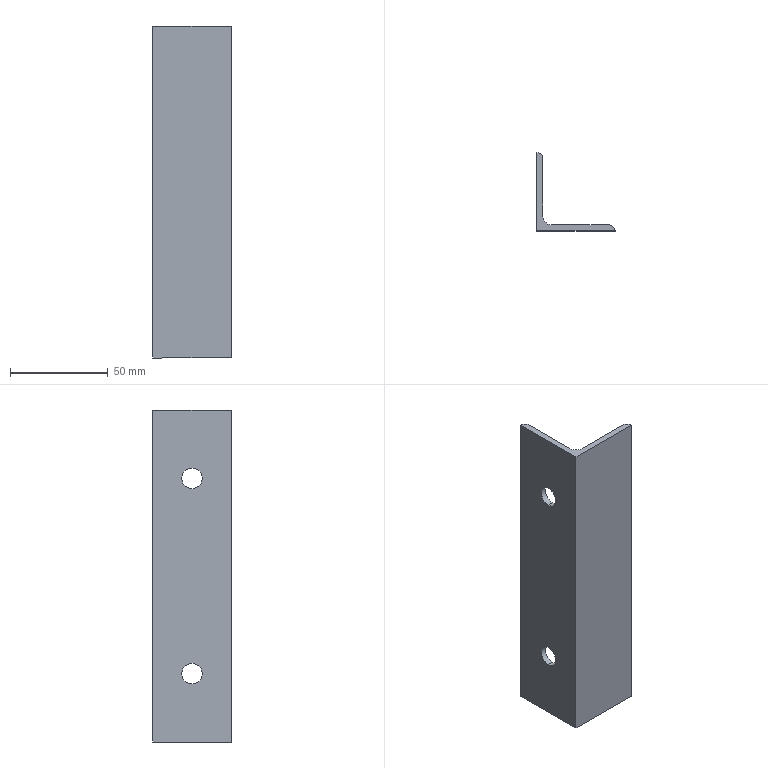Part | SolidWorks | features BaseBody 1 | 1 solid | 13 faces | box 40 x 40 x 170 mm | volume 38833 mm3 | cylinder 7 | plane 6 | commonest cylinder face diameters 10.5 x4 6 x2 9 x1
STEP:
#1=CARTESIAN_POINT('',(3.,20.,-55.25));
#2=VERTEX_POINT('',#1);
#3=CARTESIAN_POINT('',(0.,20.,-55.25));
#4=VERTEX_POINT('',#3);
#5=CARTESIAN_POINT('',(10.,20.,-55.25));
#6=DIRECTION('',(-1.,0.,0.));
#7=VECTOR('',#6,1000.);
#8=LINE('',#5,#7);
#9=EDGE_CURVE('',#2,#4,#8,.T.);
#10=ORIENTED_EDGE('',*,*,#9,.F.);
#11=CARTESIAN_POINT('',(3.,20.,-44.75));
#12=VERTEX_POINT('',#11);
#13=CARTESIAN_POINT('',(3.,20.,-50.));
#14=DIRECTION('',(-1.,0.,0.));
#15=DIRECTION('',(0.,-1.,0.));
#16=AXIS2_PLACEMENT_3D('',#13,#14,#15);
#17=CIRCLE('',#16,5.25);
#18=EDGE_CURVE('',#12,#2,#17,.T.);
#19=ORIENTED_EDGE('',*,*,#18,.F.);
#20=CARTESIAN_POINT('',(0.,20.,-44.75));
#21=VERTEX_POINT('',#20);
#22=CARTESIAN_POINT('',(10.,20.,-44.75));
#23=DIRECTION('',(-1.,0.,0.));
#24=VECTOR('',#23,1000.);
#25=LINE('',#22,#24);
#26=EDGE_CURVE('',#12,#21,#25,.T.);
#27=ORIENTED_EDGE('',*,*,#26,.T.);
#28=CARTESIAN_POINT('',(0.,20.,-50.));
#29=DIRECTION('',(-1.,0.,0.));
#30=DIRECTION('',(0.,0.,1.));
#31=AXIS2_PLACEMENT_3D('',#28,#29,#30);
#32=CIRCLE('',#31,5.25);
#33=EDGE_CURVE('',#21,#4,#32,.T.);
#34=ORIENTED_EDGE('',*,*,#33,.T.);
#35=EDGE_LOOP('',(#10,#19,#27,#34));
#36=FACE_OUTER_BOUND('',#35,.T.);
#37=CARTESIAN_POINT('',(10.,20.,-50.));
#38=DIRECTION('',(-1.,0.,0.));
#39=DIRECTION('',(0.,0.,1.));
#40=AXIS2_PLACEMENT_3D('',#37,#38,#39);
#41=CYLINDRICAL_SURFACE('',#40,5.25);
#42=ADVANCED_FACE('',(#36),#41,.F.);
#43=CARTESIAN_POINT('',(3.,20.,44.75));
#44=VERTEX_POINT('',#43);
#45=CARTESIAN_POINT('',(0.,20.,44.75));
#46=VERTEX_POINT('',#45);
#47=CARTESIAN_POINT('',(10.,20.,44.75));
#48=DIRECTION('',(-1.,0.,0.));
#49=VECTOR('',#48,1000.);
#50=LINE('',#47,#49);
#51=EDGE_CURVE('',#44,#46,#50,.T.);
#52=ORIENTED_EDGE('',*,*,#51,.F.);
#53=CARTESIAN_POINT('',(3.,20.,55.25));
#54=VERTEX_POINT('',#53);
#55=CARTESIAN_POINT('',(3.,20.,50.));
#56=DIRECTION('',(-1.,0.,0.));
#57=DIRECTION('',(0.,-1.,0.));
#58=AXIS2_PLACEMENT_3D('',#55,#56,#57);
#59=CIRCLE('',#58,5.25);
#60=EDGE_CURVE('',#54,#44,#59,.T.);
#61=ORIENTED_EDGE('',*,*,#60,.F.);
#62=CARTESIAN_POINT('',(0.,20.,55.25));
#63=VERTEX_POINT('',#62);
#64=CARTESIAN_POINT('',(10.,20.,55.25));
#65=DIRECTION('',(-1.,0.,0.));
#66=VECTOR('',#65,1000.);
#67=LINE('',#64,#66);
#68=EDGE_CURVE('',#54,#63,#67,.T.);
#69=ORIENTED_EDGE('',*,*,#68,.T.);
#70=CARTESIAN_POINT('',(0.,20.,50.));
#71=DIRECTION('',(-1.,0.,0.));
#72=DIRECTION('',(0.,0.,-1.));
#73=AXIS2_PLACEMENT_3D('',#70,#71,#72);
#74=CIRCLE('',#73,5.25);
#75=EDGE_CURVE('',#63,#46,#74,.T.);
#76=ORIENTED_EDGE('',*,*,#75,.T.);
#77=EDGE_LOOP('',(#52,#61,#69,#76));
#78=FACE_OUTER_BOUND('',#77,.T.);
#79=CARTESIAN_POINT('',(10.,20.,50.));
#80=DIRECTION('',(-1.,0.,0.));
#81=DIRECTION('',(0.,0.,1.));
#82=AXIS2_PLACEMENT_3D('',#79,#80,#81);
#83=CYLINDRICAL_SURFACE('',#82,5.25);
#84=ADVANCED_FACE('',(#78),#83,.F.);
#85=CARTESIAN_POINT('',(3.,37.,85.));
#86=VERTEX_POINT('',#85);
#87=CARTESIAN_POINT('',(0.,40.,85.));
#88=VERTEX_POINT('',#87);
#89=CARTESIAN_POINT('',(0.,37.,85.));
#90=DIRECTION('',(0.,0.,1.));
#91=DIRECTION('',(-1.,0.,0.));
#92=AXIS2_PLACEMENT_3D('',#89,#90,#91);
#93=CIRCLE('',#92,3.);
#94=EDGE_CURVE('',#86,#88,#93,.T.);
#95=ORIENTED_EDGE('',*,*,#94,.F.);
#96=CARTESIAN_POINT('',(3.,37.,-85.));
#97=VERTEX_POINT('',#96);
#98=CARTESIAN_POINT('',(3.,37.,85.));
#99=DIRECTION('',(0.,0.,1.));
#100=VECTOR('',#99,1000.);
#101=LINE('',#98,#100);
#102=EDGE_CURVE('',#97,#86,#101,.T.);
#103=ORIENTED_EDGE('',*,*,#102,.F.);
#104=CARTESIAN_POINT('',(0.,40.,-85.));
#105=VERTEX_POINT('',#104);
#106=CARTESIAN_POINT('',(0.,37.,-85.));
#107=DIRECTION('',(0.,0.,-1.));
#108=DIRECTION('',(-1.,0.,0.));
#109=AXIS2_PLACEMENT_3D('',#106,#107,#108);
#110=CIRCLE('',#109,3.);
#111=EDGE_CURVE('',#105,#97,#110,.T.);
#112=ORIENTED_EDGE('',*,*,#111,.F.);
#113=CARTESIAN_POINT('',(0.,40.,85.));
#114=DIRECTION('',(0.,0.,-1.));
#115=VECTOR('',#114,1000.);
#116=LINE('',#113,#115);
#117=EDGE_CURVE('',#88,#105,#116,.T.);
#118=ORIENTED_EDGE('',*,*,#117,.F.);
#119=EDGE_LOOP('',(#95,#103,#112,#118));
#120=FACE_OUTER_BOUND('',#119,.T.);
#121=CARTESIAN_POINT('',(0.,37.,85.));
#122=DIRECTION('',(0.,0.,-1.));
#123=DIRECTION('',(-1.,0.,0.));
#124=AXIS2_PLACEMENT_3D('',#121,#122,#123);
#125=CYLINDRICAL_SURFACE('',#124,3.);
#126=ADVANCED_FACE('',(#120),#125,.T.);
#127=CARTESIAN_POINT('',(40.,0.,85.));
#128=VERTEX_POINT('',#127);
#129=CARTESIAN_POINT('',(37.,3.,85.));
#130=VERTEX_POINT('',#129);
#131=CARTESIAN_POINT('',(37.,0.,85.));
#132=DIRECTION('',(0.,0.,1.));
#133=DIRECTION('',(-1.,0.,0.));
#134=AXIS2_PLACEMENT_3D('',#131,#132,#133);
#135=CIRCLE('',#134,3.);
#136=EDGE_CURVE('',#128,#130,#135,.T.);
#137=ORIENTED_EDGE('',*,*,#136,.F.);
#138=CARTESIAN_POINT('',(40.,0.,-85.));
#139=VERTEX_POINT('',#138);
#140=CARTESIAN_POINT('',(40.,0.,85.));
#141=DIRECTION('',(0.,0.,-1.));
#142=VECTOR('',#141,1000.);
#143=LINE('',#140,#142);
#144=EDGE_CURVE('',#128,#139,#143,.T.);
#145=ORIENTED_EDGE('',*,*,#144,.T.);
#146=CARTESIAN_POINT('',(37.,3.,-85.));
#147=VERTEX_POINT('',#146);
#148=CARTESIAN_POINT('',(37.,0.,-85.));
#149=DIRECTION('',(0.,0.,-1.));
#150=DIRECTION('',(-1.,0.,0.));
#151=AXIS2_PLACEMENT_3D('',#148,#149,#150);
#152=CIRCLE('',#151,3.);
#153=EDGE_CURVE('',#147,#139,#152,.T.);
#154=ORIENTED_EDGE('',*,*,#153,.F.);
#155=CARTESIAN_POINT('',(37.,3.,85.));
#156=DIRECTION('',(0.,0.,-1.));
#157=VECTOR('',#156,1000.);
#158=LINE('',#155,#157);
#159=EDGE_CURVE('',#130,#147,#158,.T.);
#160=ORIENTED_EDGE('',*,*,#159,.F.);
#161=EDGE_LOOP('',(#137,#145,#154,#160));
#162=FACE_OUTER_BOUND('',#161,.T.);
#163=CARTESIAN_POINT('',(37.,0.,85.));
#164=DIRECTION('',(0.,0.,-1.));
#165=DIRECTION('',(-1.,0.,0.));
#166=AXIS2_PLACEMENT_3D('',#163,#164,#165);
#167=CYLINDRICAL_SURFACE('',#166,3.);
#168=ADVANCED_FACE('',(#162),#167,.T.);
#169=CARTESIAN_POINT('',(7.5,3.,85.));
#170=VERTEX_POINT('',#169);
#171=CARTESIAN_POINT('',(3.,7.5,85.));
#172=VERTEX_POINT('',#171);
#173=CARTESIAN_POINT('',(7.5,7.5,85.));
#174=DIRECTION('',(0.,0.,-1.));
#175=DIRECTION('',(-1.,0.,0.));
#176=AXIS2_PLACEMENT_3D('',#173,#174,#175);
#177=CIRCLE('',#176,4.5);
#178=EDGE_CURVE('',#170,#172,#177,.T.);
#179=ORIENTED_EDGE('',*,*,#178,.F.);
#180=CARTESIAN_POINT('',(7.5,3.,-85.));
#181=VERTEX_POINT('',#180);
#182=CARTESIAN_POINT('',(7.5,3.,85.));
#183=DIRECTION('',(0.,0.,1.));
#184=VECTOR('',#183,1000.);
#185=LINE('',#182,#184);
#186=EDGE_CURVE('',#181,#170,#185,.T.);
#187=ORIENTED_EDGE('',*,*,#186,.F.);
#188=CARTESIAN_POINT('',(3.,7.5,-85.));
#189=VERTEX_POINT('',#188);
#190=CARTESIAN_POINT('',(7.5,7.5,-85.));
#191=DIRECTION('',(0.,0.,1.));
#192=DIRECTION('',(-1.,0.,0.));
#193=AXIS2_PLACEMENT_3D('',#190,#191,#192);
#194=CIRCLE('',#193,4.5);
#195=EDGE_CURVE('',#189,#181,#194,.T.);
#196=ORIENTED_EDGE('',*,*,#195,.F.);
#197=CARTESIAN_POINT('',(3.,7.5,-85.));
#198=DIRECTION('',(0.,0.,-1.));
#199=VECTOR('',#198,1000.);
#200=LINE('',#197,#199);
#201=EDGE_CURVE('',#172,#189,#200,.T.);
#202=ORIENTED_EDGE('',*,*,#201,.F.);
#203=EDGE_LOOP('',(#179,#187,#196,#202));
#204=FACE_OUTER_BOUND('',#203,.T.);
#205=CARTESIAN_POINT('',(7.5,7.5,85.));
#206=DIRECTION('',(0.,0.,1.));
#207=DIRECTION('',(1.,0.,0.));
#208=AXIS2_PLACEMENT_3D('',#205,#206,#207);
#209=CYLINDRICAL_SURFACE('',#208,4.5);
#210=ADVANCED_FACE('',(#204),#209,.F.);
#211=CARTESIAN_POINT('',(3.,3.,-85.));
#212=DIRECTION('',(-1.,0.,0.));
#213=VECTOR('',#212,1000.);
#214=LINE('',#211,#213);
#215=EDGE_CURVE('',#147,#181,#214,.T.);
#216=ORIENTED_EDGE('',*,*,#215,.F.);
#217=ORIENTED_EDGE('',*,*,#153,.T.);
#218=CARTESIAN_POINT('',(0.,0.,-85.));
#219=VERTEX_POINT('',#218);
#220=CARTESIAN_POINT('',(0.,0.,-85.));
#221=DIRECTION('',(1.,0.,0.));
#222=VECTOR('',#221,1000.);
#223=LINE('',#220,#222);
#224=EDGE_CURVE('',#219,#139,#223,.T.);
#225=ORIENTED_EDGE('',*,*,#224,.F.);
#226=CARTESIAN_POINT('',(0.,0.,-85.));
#227=DIRECTION('',(0.,-1.,0.));
#228=VECTOR('',#227,1000.);
#229=LINE('',#226,#228);
#230=EDGE_CURVE('',#105,#219,#229,.T.);
#231=ORIENTED_EDGE('',*,*,#230,.F.);
#232=ORIENTED_EDGE('',*,*,#111,.T.);
#233=CARTESIAN_POINT('',(3.,40.,-85.));
#234=DIRECTION('',(0.,1.,0.));
#235=VECTOR('',#234,1000.);
#236=LINE('',#233,#235);
#237=EDGE_CURVE('',#189,#97,#236,.T.);
#238=ORIENTED_EDGE('',*,*,#237,.F.);
#239=ORIENTED_EDGE('',*,*,#195,.T.);
#240=EDGE_LOOP('',(#216,#217,#225,#231,#232,#238,#239));
#241=FACE_OUTER_BOUND('',#240,.T.);
#242=CARTESIAN_POINT('',(0.,0.,-85.));
#243=DIRECTION('',(0.,0.,-1.));
#244=DIRECTION('',(0.,-1.,0.));
#245=AXIS2_PLACEMENT_3D('',#242,#243,#244);
#246=PLANE('',#245);
#247=ADVANCED_FACE('',(#241),#246,.T.);
#248=CARTESIAN_POINT('',(0.,0.,85.));
#249=VERTEX_POINT('',#248);
#250=CARTESIAN_POINT('',(0.,0.,85.));
#251=DIRECTION('',(1.,0.,0.));
#252=VECTOR('',#251,1000.);
#253=LINE('',#250,#252);
#254=EDGE_CURVE('',#249,#128,#253,.T.);
#255=ORIENTED_EDGE('',*,*,#254,.T.);
#256=ORIENTED_EDGE('',*,*,#136,.T.);
#257=CARTESIAN_POINT('',(3.,3.,85.));
#258=DIRECTION('',(-1.,0.,0.));
#259=VECTOR('',#258,1000.);
#260=LINE('',#257,#259);
#261=EDGE_CURVE('',#130,#170,#260,.T.);
#262=ORIENTED_EDGE('',*,*,#261,.T.);
#263=ORIENTED_EDGE('',*,*,#178,.T.);
#264=CARTESIAN_POINT('',(3.,40.,85.));
#265=DIRECTION('',(0.,1.,0.));
#266=VECTOR('',#265,1000.);
#267=LINE('',#264,#266);
#268=EDGE_CURVE('',#172,#86,#267,.T.);
#269=ORIENTED_EDGE('',*,*,#268,.T.);
#270=ORIENTED_EDGE('',*,*,#94,.T.);
#271=CARTESIAN_POINT('',(0.,0.,85.));
#272=DIRECTION('',(0.,-1.,0.));
#273=VECTOR('',#272,1000.);
#274=LINE('',#271,#273);
#275=EDGE_CURVE('',#88,#249,#274,.T.);
#276=ORIENTED_EDGE('',*,*,#275,.T.);
#277=EDGE_LOOP('',(#255,#256,#262,#263,#269,#270,#276));
#278=FACE_OUTER_BOUND('',#277,.T.);
#279=CARTESIAN_POINT('',(0.,0.,85.));
#280=DIRECTION('',(0.,0.,-1.));
#281=DIRECTION('',(0.,-1.,0.));
#282=AXIS2_PLACEMENT_3D('',#279,#280,#281);
#283=PLANE('',#282);
#284=ADVANCED_FACE('',(#278),#283,.F.);
#285=ORIENTED_EDGE('',*,*,#60,.T.);
#286=CARTESIAN_POINT('',(3.,20.,50.));
#287=DIRECTION('',(-1.,0.,0.));
#288=DIRECTION('',(0.,-1.,0.));
#289=AXIS2_PLACEMENT_3D('',#286,#287,#288);
#290=CIRCLE('',#289,5.25);
#291=EDGE_CURVE('',#44,#54,#290,.T.);
#292=ORIENTED_EDGE('',*,*,#291,.T.);
#293=EDGE_LOOP('',(#285,#292));
#294=FACE_BOUND('',#293,.T.);
#295=ORIENTED_EDGE('',*,*,#18,.T.);
#296=CARTESIAN_POINT('',(3.,20.,-50.));
#297=DIRECTION('',(-1.,0.,0.));
#298=DIRECTION('',(0.,-1.,0.));
#299=AXIS2_PLACEMENT_3D('',#296,#297,#298);
#300=CIRCLE('',#299,5.25);
#301=EDGE_CURVE('',#2,#12,#300,.T.);
#302=ORIENTED_EDGE('',*,*,#301,.T.);
#303=EDGE_LOOP('',(#295,#302));
#304=FACE_BOUND('',#303,.T.);
#305=ORIENTED_EDGE('',*,*,#237,.T.);
#306=ORIENTED_EDGE('',*,*,#102,.T.);
#307=ORIENTED_EDGE('',*,*,#268,.F.);
#308=ORIENTED_EDGE('',*,*,#201,.T.);
#309=EDGE_LOOP('',(#305,#306,#307,#308));
#310=FACE_OUTER_BOUND('',#309,.T.);
#311=CARTESIAN_POINT('',(3.,40.,85.));
#312=DIRECTION('',(-1.,0.,0.));
#313=DIRECTION('',(0.,1.,0.));
#314=AXIS2_PLACEMENT_3D('',#311,#312,#313);
#315=PLANE('',#314);
#316=ADVANCED_FACE('',(#294,#304,#310),#315,.F.);
#317=ORIENTED_EDGE('',*,*,#261,.F.);
#318=ORIENTED_EDGE('',*,*,#159,.T.);
#319=ORIENTED_EDGE('',*,*,#215,.T.);
#320=ORIENTED_EDGE('',*,*,#186,.T.);
#321=EDGE_LOOP('',(#317,#318,#319,#320));
#322=FACE_OUTER_BOUND('',#321,.T.);
#323=CARTESIAN_POINT('',(3.,3.,85.));
#324=DIRECTION('',(0.,-1.,0.));
#325=DIRECTION('',(0.,0.,-1.));
#326=AXIS2_PLACEMENT_3D('',#323,#324,#325);
#327=PLANE('',#326);
#328=ADVANCED_FACE('',(#322),#327,.F.);
#329=ORIENTED_EDGE('',*,*,#224,.T.);
#330=ORIENTED_EDGE('',*,*,#144,.F.);
#331=ORIENTED_EDGE('',*,*,#254,.F.);
#332=CARTESIAN_POINT('',(0.,0.,85.));
#333=DIRECTION('',(0.,0.,-1.));
#334=VECTOR('',#333,1000.);
#335=LINE('',#332,#334);
#336=EDGE_CURVE('',#249,#219,#335,.T.);
#337=ORIENTED_EDGE('',*,*,#336,.T.);
#338=EDGE_LOOP('',(#329,#330,#331,#337));
#339=FACE_OUTER_BOUND('',#338,.T.);
#340=CARTESIAN_POINT('',(0.,0.,85.));
#341=DIRECTION('',(0.,1.,0.));
#342=DIRECTION('',(1.,0.,0.));
#343=AXIS2_PLACEMENT_3D('',#340,#341,#342);
#344=PLANE('',#343);
#345=ADVANCED_FACE('',(#339),#344,.F.);
#346=ORIENTED_EDGE('',*,*,#75,.F.);
#347=CARTESIAN_POINT('',(0.,20.,50.));
#348=DIRECTION('',(-1.,0.,0.));
#349=DIRECTION('',(0.,0.,-1.));
#350=AXIS2_PLACEMENT_3D('',#347,#348,#349);
#351=CIRCLE('',#350,5.25);
#352=EDGE_CURVE('',#46,#63,#351,.T.);
#353=ORIENTED_EDGE('',*,*,#352,.F.);
#354=EDGE_LOOP('',(#346,#353));
#355=FACE_BOUND('',#354,.T.);
#356=ORIENTED_EDGE('',*,*,#33,.F.);
#357=CARTESIAN_POINT('',(0.,20.,-50.));
#358=DIRECTION('',(-1.,0.,0.));
#359=DIRECTION('',(0.,0.,1.));
#360=AXIS2_PLACEMENT_3D('',#357,#358,#359);
#361=CIRCLE('',#360,5.25);
#362=EDGE_CURVE('',#4,#21,#361,.T.);
#363=ORIENTED_EDGE('',*,*,#362,.F.);
#364=EDGE_LOOP('',(#356,#363));
#365=FACE_BOUND('',#364,.T.);
#366=ORIENTED_EDGE('',*,*,#230,.T.);
#367=ORIENTED_EDGE('',*,*,#336,.F.);
#368=ORIENTED_EDGE('',*,*,#275,.F.);
#369=ORIENTED_EDGE('',*,*,#117,.T.);
#370=EDGE_LOOP('',(#366,#367,#368,#369));
#371=FACE_OUTER_BOUND('',#370,.T.);
#372=CARTESIAN_POINT('',(0.,0.,85.));
#373=DIRECTION('',(1.,0.,0.));
#374=DIRECTION('',(0.,1.,0.));
#375=AXIS2_PLACEMENT_3D('',#372,#373,#374);
#376=PLANE('',#375);
#377=ADVANCED_FACE('',(#355,#365,#371),#376,.F.);
#378=ORIENTED_EDGE('',*,*,#291,.F.);
#379=ORIENTED_EDGE('',*,*,#51,.T.);
#380=ORIENTED_EDGE('',*,*,#352,.T.);
#381=ORIENTED_EDGE('',*,*,#68,.F.);
#382=EDGE_LOOP('',(#378,#379,#380,#381));
#383=FACE_OUTER_BOUND('',#382,.T.);
#384=CARTESIAN_POINT('',(10.,20.,50.));
#385=DIRECTION('',(-1.,0.,0.));
#386=DIRECTION('',(0.,0.,1.));
#387=AXIS2_PLACEMENT_3D('',#384,#385,#386);
#388=CYLINDRICAL_SURFACE('',#387,5.25);
#389=ADVANCED_FACE('',(#383),#388,.F.);
#390=ORIENTED_EDGE('',*,*,#301,.F.);
#391=ORIENTED_EDGE('',*,*,#9,.T.);
#392=ORIENTED_EDGE('',*,*,#362,.T.);
#393=ORIENTED_EDGE('',*,*,#26,.F.);
#394=EDGE_LOOP('',(#390,#391,#392,#393));
#395=FACE_OUTER_BOUND('',#394,.T.);
#396=CARTESIAN_POINT('',(10.,20.,-50.));
#397=DIRECTION('',(-1.,0.,0.));
#398=DIRECTION('',(0.,0.,1.));
#399=AXIS2_PLACEMENT_3D('',#396,#397,#398);
#400=CYLINDRICAL_SURFACE('',#399,5.25);
#401=ADVANCED_FACE('',(#395),#400,.F.);
#402=CLOSED_SHELL('',(#42,#84,#126,#168,#210,#247,#284,#316,#328,#345,#377,#389,#401));
#403=MANIFOLD_SOLID_BREP('',#402);
#404=CARTESIAN_POINT('',(0.,0.,0.));
#405=DIRECTION('',(0.,0.,1.));
#406=DIRECTION('',(1.,0.,0.));
#407=AXIS2_PLACEMENT_3D('',#404,#405,#406);
#408=(LENGTH_UNIT()NAMED_UNIT(*)SI_UNIT(.MILLI.,.METRE.));
#409=UNCERTAINTY_MEASURE_WITH_UNIT(LENGTH_MEASURE(0.00001),#408,'','');
#410=(NAMED_UNIT(*)PLANE_ANGLE_UNIT()SI_UNIT($,.RADIAN.));
#411=(NAMED_UNIT(*)SI_UNIT($,.STERADIAN.)SOLID_ANGLE_UNIT());
#412=(GEOMETRIC_REPRESENTATION_CONTEXT(3)GLOBAL_UNCERTAINTY_ASSIGNED_CONTEXT((#409))GLOBAL_UNIT_ASSIGNED_CONTEXT((#408,#410,#411))REPRESENTATION_CONTEXT('',''));
#413=ADVANCED_BREP_SHAPE_REPRESENTATION('',(#403,#407),#412);